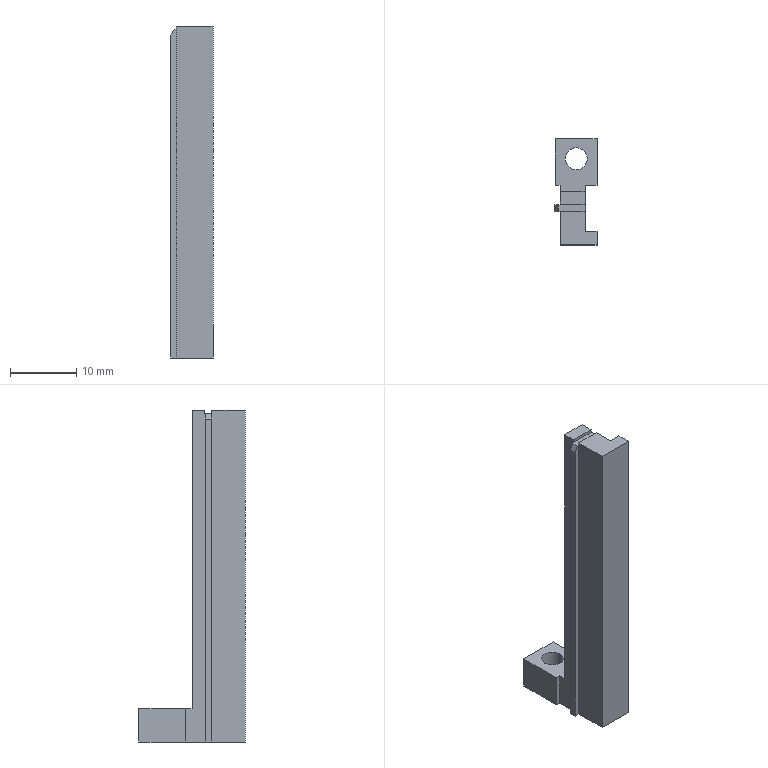Part | STEP file | Rivet push rod_Default | 1 solid | 25 faces | box 6.34 x 16 x 50 mm | volume 1914 mm3 | plane 23 | cylinder 2 | commonest cylinder face diameters 3.3 x2